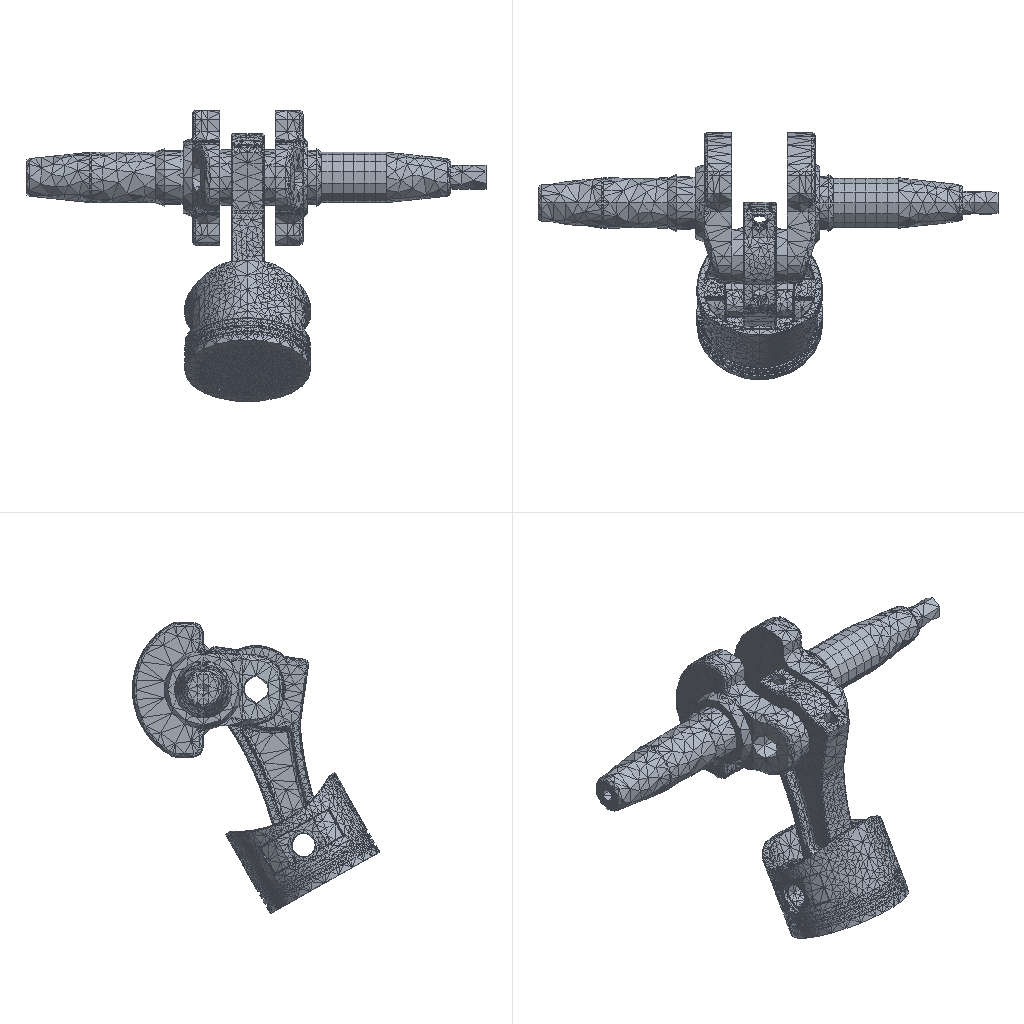Simulation study | ansys workbench
Set-up summary:
category,name,step,type,value,unit,region
solver,ansys_workbench
units,mm-N-s-tonne (MPa),,stated,"/units,MPA"
analysis,LS1,,static
load_step,LS1,LS1,static,nsubst=1; time=1
mesh,nodes,,,69706
mesh,elements,,,40599
element_type,SOLID187,,,38152
element_type,SURF154,,,1167
element_type,TARGE170,,,565
element_type,CONTA174,,,565
element_type,SOLID186,,,150
material,42Cr,,E,200000,tonne s^-2 mm^-1
material,42Cr,,nu,0.3
material,42Cr,,density,7.85e-09,tonne mm^-3
material,42Cr,,conductivity,60.5,tonne mm s^-3 C^-1
material,42Cr,,specific_heat,4.34e+08,mm^2 s^-2 C^-1
material,42Cr,,cte,1.2e-05,C^-1
material,42Cr,,permeability,10000
material,42Cr,,resistivity,0.00017,ohm mm
load,Define Force Using Surface Effect Elements,LS1,surface-effect pres face 1,0.5577,,SURF154 #13
bc,Fixed Supports,model,fixed,[dofs=ALL],,_FIXEDSU
contact,Contact Region,,bonded (always),element=CONTA174
contact,Contact Region 2,,bonded (always),element=CONTA174
contact,Contact Region 3,,bonded (always),element=CONTA174
named_set,_FIXEDSU,,node,2171
Ansys APDL input file, long lists of numbers shortened:
/batch
/config,noeldb,1     ! force off writing results to database
*get,_wallstrt,active,,time,wall
! ANSYS input file written by Workbench version 2022 R1
! File used for geometry attach:
/title,wbnew--____ (B5)
! ****** Begin Custom Load Command Snippet ******
/COM, ACT Extensions:
/COM,     LSDYNA, 2021.1
/COM,
! ****** End   Custom Load Command Snippet ******
*DIM,_wb_ProjectScratch_dir,string,248
_wb_ProjectScratch_dir(1) = ''
*DIM,_wb_SolverFiles_dir,string,248
_wb_SolverFiles_dir(1) = ''
*DIM,_wb_userfiles_dir,string,248
_wb_userfiles_dir(1) = ''
/com,--- Data in consistent NMM units. See Solving Units in the help system for more information.
/units,MPA
/nopr
/wb,file,start              !  signify a WB generated input file
/prep7
! Turn off shape checking because checks already performed inside WB mesher.
! See help system for more information.
SHPP,OFF,,NOWARN
/nolist
etcon,set             ! allow ANSYS to choose best KEYOP's for 180x elements, resets any applicable keyopt to MAPDL defaults
/com,*********** Nodes for the whole assembly ***********
nblock,3,,76676
(1i9,3e20.9e3)
        1     9.804117852E+01     4.011351533E+00    -7.980678705E-01
! (69705 more lines like these left out)
-1
/wb,elem,start            !  set before creation of elements
/com,*********** Elements for Body 1 "Crank shaft|NONE" ***********
et,1,186
keyo,1,2,1          ! set full integration on SOLID186
eblock,19,solid,,150
(19i9)
        1        1        1        1        0        0        0        0       20        0        1        1        6       56       16      114      113      103      111
! (299 more lines like these left out)
-1
/com,*********** Elements for Body 2 "Crank shaft|NONE[2]" ***********
et,2,187
eblock,19,solid,,891
(19i9)
        2        2        2        2        0        0        0        0       10        0      669     1893     2107     1998     2048     2495     3078     2492     2494
! (1781 more lines like these left out)
-1
/com,*********** Elements for Body 3 "Crank shaft|NONE[3]" ***********
et,3,187
eblock,19,solid,,3251
(19i9)
        3        3        3        3        0        0        0        0       10        0     1560     4349     4542     4469     4534     9241     9703     9237     9240
! (6501 more lines like these left out)
-1
/com,*********** Elements for Body 4 "Crank shaft|NONE[4]" ***********
et,4,187
eblock,19,solid,,518
(19i9)
        4        4        4        4        0        0        0        0       10        0      151      857      869      889     1001     1191     1280     1192     1200
! (1035 more lines like these left out)
-1
/com,*********** Elements for Body 5 "Cnrod|NONE" ***********
et,5,187
eblock,19,solid,,7843
(19i9)
        5        5        5        5        0        0        0        0       10        0     4811    10215    11725    12028    11889    15510    23428    15513    15511
! (15685 more lines like these left out)
-1
/com,*********** Elements for Body 6 "Piston|NONE" ***********
et,6,187
eblock,19,solid,,25649
(19i9)
        6        6        6        6        0        0        0        0       10        0    12654    29657    30685    31222    31214    64657    69195    64660    64659
! (51297 more lines like these left out)
-1
/wb,elem,end               !  done creating elements
/com,*********** Send User Defined Coordinate System(s) ***********
csys,0
toffst,273.15,  ! Temperature offset from absolute zero
/com,*********** Set Reference Temperature ***********
tref,22.
/wb,mat,start              !  starting to send materials
/com,*********** Send Materials ***********
Temperature = 'TEMP' ! Temperature
MP,DENS,1,7.85e-09,	! tonne mm^-3
MP,ALPX,1,1.2e-05,	! C^-1
MP,C,1,434000000,	! mm^2 s^-2 C^-1
MP,KXX,1,60.5,	! tonne mm s^-3 C^-1
MP,RSVX,1,0.00017,	! ohm mm
MP,EX,1,200000,	! tonne s^-2 mm^-1
MP,NUXY,1,0.3,
MP,MURX,1,10000,
Temperature = 'TEMP' ! Temperature
MP,DENS,2,7.85e-09,	! tonne mm^-3
MP,ALPX,2,1.2e-05,	! C^-1
MP,C,2,434000000,	! mm^2 s^-2 C^-1
MP,KXX,2,60.5,	! tonne mm s^-3 C^-1
MP,RSVX,2,0.00017,	! ohm mm
MP,EX,2,200000,	! tonne s^-2 mm^-1
MP,NUXY,2,0.3,
MP,MURX,2,10000,
Temperature = 'TEMP' ! Temperature
MP,DENS,3,7.85e-09,	! tonne mm^-3
MP,ALPX,3,1.2e-05,	! C^-1
MP,C,3,434000000,	! mm^2 s^-2 C^-1
MP,KXX,3,60.5,	! tonne mm s^-3 C^-1
MP,RSVX,3,0.00017,	! ohm mm
MP,EX,3,200000,	! tonne s^-2 mm^-1
MP,NUXY,3,0.3,
MP,MURX,3,10000,
Temperature = 'TEMP' ! Temperature
MP,DENS,4,7.85e-09,	! tonne mm^-3
MP,ALPX,4,1.2e-05,	! C^-1
MP,C,4,434000000,	! mm^2 s^-2 C^-1
MP,KXX,4,60.5,	! tonne mm s^-3 C^-1
MP,RSVX,4,0.00017,	! ohm mm
MP,EX,4,200000,	! tonne s^-2 mm^-1
MP,NUXY,4,0.3,
MP,MURX,4,10000,
Temperature = 'TEMP' ! Temperature
MP,DENS,5,7.85e-09,	! tonne mm^-3
MP,ALPX,5,1.2e-05,	! C^-1
MP,C,5,434000000,	! mm^2 s^-2 C^-1
MP,KXX,5,60.5,	! tonne mm s^-3 C^-1
MP,RSVX,5,0.00017,	! ohm mm
MP,EX,5,200000,	! tonne s^-2 mm^-1
MP,NUXY,5,0.3,
MP,MURX,5,10000,
Temperature = 'TEMP' ! Temperature
MP,DENS,6,7.85e-09,	! tonne mm^-3
MP,ALPX,6,1.2e-05,	! C^-1
MP,C,6,434000000,	! mm^2 s^-2 C^-1
MP,KXX,6,60.5,	! tonne mm s^-3 C^-1
MP,RSVX,6,0.00017,	! ohm mm
MP,EX,6,200000,	! tonne s^-2 mm^-1
MP,NUXY,6,0.3,
MP,MURX,6,10000,
/wb,mat,end                !  done sending materials
!************************* Model Summary ********************
!Crank shaft|NONE,	42Cr,	matid,	1
!Crank shaft|NONE[2],	42Cr,	matid,	2
!Crank shaft|NONE[3],	42Cr,	matid,	3
!Crank shaft|NONE[4],	42Cr,	matid,	4
!Cnrod|NONE,	42Cr,	matid,	5
!Piston|NONE,	42Cr,	matid,	6
!************************* End Model Summary ********************
! get the diagonal of the bounding box. Needed later for other things
*get,_xmin,node,,mnloc,x
*get,_ymin,node,,mnloc,y
*get,_zmin,node,,mnloc,z
*get,_xmax,node,,mxloc,x
*get,_ymax,node,,mxloc,y
*get,_zmax,node,,mxloc,z
_ASMDIAG=(_xmax-_xmin)*(_xmax-_xmin)+(_ymax-_ymin)*(_ymax-_ymin)+(_zmax-_zmin)*(_zmax-_zmin)
_ASMDIAG=SQRT(_ASMDIAG)
/wb,contact,start          !  starting to send contact
/com,*********** Create Contact "接触区域" ***********
/com,            Real Constant Set For Above Contact Is 8 & 7
*set,tid,8
*set,cid,7
r,tid
r,cid
et,tid,170
et,cid,174
eblock,10,,,25
(15i9)
    55723        8        8        8        0      113      103      111      114      588      586      602      603
! (24 more lines like these left out)
-1
eblock,10,,,25
(15i9)
    55748        7        7        7        0      113      103      111      114      588      586      602      603
! (24 more lines like these left out)
-1
eblock,10,,,12
(15i9)
    55773        7        8        7        0      879      971      880      880     1325     1330      880     1322
! (11 more lines like these left out)
-1
eblock,10,,,12
(15i9)
    55785        8        7        8        0      879      971      880      880     1325     1330      880     1322
! (11 more lines like these left out)
-1
keyo,cid,8,2               ! auto create asymmetric contact (from Program Controlled setting)
keyo,cid,10,0              ! adjust contact stiffness each NR iteration (from Program Controlled setting)
keyo,cid,12,5              ! bonded always
keyo,cid,18,1              ! small sliding turned on by application
keyo,cid,2,0               ! augmented Lagrange (from Program Controlled setting)
keyo,cid,4,0               ! on Gauss point (from Program Controlled setting)
keyo,cid,9,1               ! ignore initial gaps/penetration
keyo,cid,7,0               ! No Prediction
rmod,tid,3,10.      ! FKN
rmod,tid,5,0.       ! ICONT
rmod,tid,6,0.       ! PINB
rmod,tid,10,0.      ! CNOF
rmod,tid,12,0.      ! FKT
rmod,tid,36,73      ! WB DSID
rmod,cid,3,10.      ! FKN
rmod,cid,5,0.       ! ICONT
rmod,cid,6,0.       ! PINB
rmod,cid,10,0.      ! CNOF
rmod,cid,12,0.      ! FKT
rmod,cid,36,73      ! WB DSID
/com,*********** Create Contact "接触区域 2" ***********
/com,            Real Constant Set For Above Contact Is 10 & 9
*set,tid,10
*set,cid,9
r,tid
r,cid
et,tid,170
et,cid,174
eblock,10,,,12
(15i9)
    55797       10       10       10        0     1880     1874     1885     1885     2380     2381     1885     2412
! (11 more lines like these left out)
-1
eblock,10,,,12
(15i9)
    55809        9        9        9        0     1880     1874     1885     1885     2380     2381     1885     2412
! (11 more lines like these left out)
-1
eblock,10,,,10
(15i9)
    55821        9       10        9        0     4085     3706     3712     3712     6137     6135     3712     6192
! (9 more lines like these left out)
-1
eblock,10,,,10
(15i9)
    55831       10        9       10        0     4085     3706     3712     3712     6137     6135     3712     6192
! (9 more lines like these left out)
-1
keyo,cid,8,2               ! auto create asymmetric contact (from Program Controlled setting)
keyo,cid,10,0              ! adjust contact stiffness each NR iteration (from Program Controlled setting)
keyo,cid,12,5              ! bonded always
keyo,cid,18,1              ! small sliding turned on by application
keyo,cid,2,0               ! augmented Lagrange (from Program Controlled setting)
keyo,cid,4,0               ! on Gauss point (from Program Controlled setting)
keyo,cid,9,1               ! ignore initial gaps/penetration
keyo,cid,7,0               ! No Prediction
rmod,tid,3,10.      ! FKN
rmod,tid,5,0.       ! ICONT
rmod,tid,6,0.       ! PINB
rmod,tid,10,0.      ! CNOF
rmod,tid,12,0.      ! FKT
rmod,tid,36,76      ! WB DSID
rmod,cid,3,10.      ! FKN
rmod,cid,5,0.       ! ICONT
rmod,cid,6,0.       ! PINB
rmod,cid,10,0.      ! CNOF
rmod,cid,12,0.      ! FKT
rmod,cid,36,76      ! WB DSID
/com,*********** Create Contact "接触区域 3" ***********
/com,            Real Constant Set For Above Contact Is 12 & 11
*set,tid,12
*set,cid,11
r,tid
r,cid
et,tid,170
et,cid,174
eblock,10,,,78
(15i9)
    55841       12       12       12        0     4163     4305     4301     4301     8622     9038     4301     8621
! (77 more lines like these left out)
-1
eblock,10,,,78
(15i9)
    55919       11       11       11        0     4163     4305     4301     4301     8622     9038     4301     8621
! (77 more lines like these left out)
-1
eblock,10,,,428
(15i9)
    55997       11       12       11        0     9871     9869    10375    10375    12824    12825    10375    12844
! (427 more lines like these left out)
-1
eblock,10,,,428
(15i9)
    56425       12       11       12        0     9871     9869    10375    10375    12824    12825    10375    12844
! (427 more lines like these left out)
-1
keyo,cid,8,2               ! auto create asymmetric contact (from Program Controlled setting)
keyo,cid,10,0              ! adjust contact stiffness each NR iteration (from Program Controlled setting)
keyo,cid,12,5              ! bonded always
keyo,cid,18,1              ! small sliding turned on by application
keyo,cid,2,0               ! augmented Lagrange (from Program Controlled setting)
keyo,cid,4,0               ! on Gauss point (from Program Controlled setting)
keyo,cid,9,1               ! ignore initial gaps/penetration
keyo,cid,7,0               ! No Prediction
rmod,tid,3,10.      ! FKN
rmod,tid,5,0.       ! ICONT
rmod,tid,6,0.       ! PINB
rmod,tid,10,0.      ! CNOF
rmod,tid,12,0.      ! FKT
rmod,tid,36,79      ! WB DSID
rmod,cid,3,10.      ! FKN
rmod,cid,5,0.       ! ICONT
rmod,cid,6,0.       ! PINB
rmod,cid,10,0.      ! CNOF
rmod,cid,12,0.      ! FKT
rmod,cid,36,79      ! WB DSID
nsel,all
esel,all
/wb,contact,end            !  done creating contacts
/golist
/wb,load,start             !  starting to send loads
/com,*********** Fixed Supports ***********
CMBLOCK,_FIXEDSU,NODE,     2171
(8i10)
       134       135       136       137       138       139       140       141
! (271 more lines like these left out)
cmsel,s,_FIXEDSU
d,all,all
nsel,all
/com,*********** Define Force Using Surface Effect Elements ***********
local,12,0,0.,0.,0.,0.,0.,0.
csys,0
et,13,154
eblock,10,,,1167
(15i9)
    56853       13       13       13       12     3886     4174     4028     4028     7410     8170     4028     7409
! (1166 more lines like these left out)
-1
esel,s,type,,13
keyop,13,2,1                ! Apply load in local coordinate system
keyop,13,7,1                ! Use original area so load is constant in large deformation
esel,all
/gst,on,on
fini
*get,_numnode,node,0,count
*get,_numelem,elem,0,count
*get, _MAXELEMNUM, elem, 0, NUM, MAX
*get, _MAXNODENUM, node, 0, NUM, MAX
*get, _MAXELEMTYPE, etyp, 0, NUM, MAX
*get, _MAXREALCONST, real, 0, NUM, MAX
/go
/wb,load,end               !  done creating loads
/com,--- Number of total nodes = %_numnode%
/com,--- Number of contact elements = 2297
/com,--- Number of spring elements = 0
/com,--- Number of bearing elements = 0
/com,--- Number of solid elements = 38302
/com,--- Number of condensed parts = 0
/com,--- Number of total elements = %_numelem%
*get,_wallbsol,active,,time,wall
/com,****************************************************************************
/com,*************************    SOLUTION       ********************************
/com,****************************************************************************
/solu
antype,0                   ! static analysis
_thickRatio=  1     ! Ratio of thick parts in the model
eqsl,pcg,1e-8,,,,,,1
cntr,print,1               ! print out contact info and also make no initial contact an error
dmpoption,emat,no             ! Don't combine emat file for DANSYS
dmpoption,esav,no             ! Don't combine esav file for DANSYS
nldiag,cont,iter           ! print out contact info each equilibrium iteration
rescontrol,,none                 ! Do not keep any restart files
/com,****************************************************
/com,******************* SOLVE FOR LS 1 OF 1 ****************
esel,s,type,,13
nsle
sfe,all,1,pres,1,0.5577
sfe,all,2,pres,1,0.
sfe,all,3,pres,1,0.
nsel,all
esel,all
/nopr
/gopr
nsub,1,1,1
time,1.
outres,erase
outres,all,none
outres,nsol,all,
outres,rsol,all
outres,eangl,all
outres,etmp,all
outres,veng,all
outres,strs,all,
outres,epel,all,
outres,eppl,all,
outres,cont,all,
! *********** WB SOLVE COMMAND ***********
! check interactive state
*get,ANSINTER_,active,,int
*if,ANSINTER_,ne,0,then
/eof
*endif
solve
/com *************** Write FE CONNECTORS *********
CEWRITE,file,ce,,INTE
/com,****************************************************
/com,*************** FINISHED SOLVE FOR LS 1 *************
*get,_wallasol,active,,time,wall
/nopr
*get,_numnode,node,0,count
*get,_numelem,elem,0,count
*get, _MAXELEMNUM, elem, 0, NUM, MAX
*get, _MAXNODENUM, node, 0, NUM, MAX,,,INTERNAL
*get, _MAXELEMTYPE, etyp, 0, NUM, MAX
*get, _MAXREALCONST, real, 0, NUM, MAX
/gopr
*get,_PCGITER,active,,solu,cgiter
/post1
xmlo,ENCODING,ISO-8859-1
xmlo,parm
/xml,parm,xml
fini
/gopr
*get,_walldone,active,,time,wall
_preptime=(_wallbsol-_wallstrt)*3600
_solvtime=(_wallasol-_wallbsol)*3600
_posttime=(_walldone-_wallasol)*3600
_totaltim=(_walldone-_wallstrt)*3600
*get,_dlbratio,active,0,solu,dlbr
*get,_combtime,active,0,solu,comb
*get,_ssmode,active,0,solu,ssmm
*get,_ndofs,active,0,solu,ndof
*get,_sol_end_time,active,0,set,time
*if,_sol_end_time,eq,1.,then
/fclean				!clean distributed files
*endif
/com,--- Total number of nodes = %_numnode%
/com,--- Total number of elements = %_numelem%
/com,--- Element load balance ratio = %_dlbratio%
/com,--- Time to combine distributed files = %_combtime%
/com,--- Sparse memory mode = %_ssmode%
/com,--- Number of DOF = %_ndofs%
/wb,file,end               ! done with WB generated input
Results summary:
result,analyses[0].index,,,1
result,analyses[0].system,,,SYS
result,analyses[0].deck,,,deck.dat
result,analyses[0].solve_status,,,completed
result,analyses[0].analysis_type,,,static
result,analyses[0].physics,,,mechanical
result,analyses[0].unit_system,,,"NMM: mm, ton, N, s, mV, mA, degC"
result,analyses[0].n_sets,,,1
result,analyses[0].load_steps[0].set,set=1,,1
result,analyses[0].load_steps[0].time_or_freq,set=1,,1
result,analyses[0].load_steps[0].max_displacement_magnitude,set=1,,0.01499
result,analyses[0].load_steps[0].max_von_mises_nodal,set=1,,42.486
result,analyses[0].load_steps[0].reaction_force_sum_xyz[1],set=1,,-5000
result,analyses[0].load_steps[0].reaction_force_sum_xyz[2],set=1,,5.34606e-06
result,analyses[0].load_steps[0].reaction_force_sum_xyz[3],set=1,,5.55179e-06